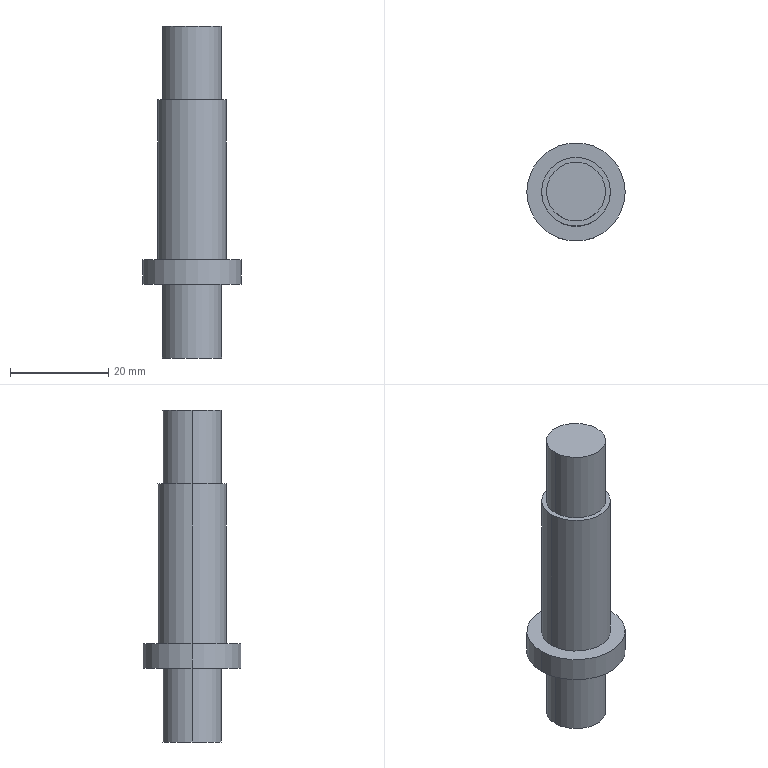Part | STEP file | Nylon handwheel shaft QY-1-37 | 1 solid | 13 faces | box 20 x 20 x 67.5 mm | volume 9967 mm3 | cylinder 8 | plane 5 | commonest cylinder face diameters 12 x4 14 x2 20 x2
STEP:
#1=CARTESIAN_POINT('',(0.,0.,0.));
#2=DIRECTION('',(0.,0.,1.));
#3=DIRECTION('',(1.,0.,0.));
#4=AXIS2_PLACEMENT_3D('',#1,#2,#3);
#5=CARTESIAN_POINT('',(-6.,0.,-20.));
#6=VERTEX_POINT('',#5);
#7=CARTESIAN_POINT('',(6.,0.,-20.));
#8=VERTEX_POINT('',#7);
#9=CARTESIAN_POINT('',(0.,0.,-20.));
#10=DIRECTION('',(0.,0.,-1.));
#11=DIRECTION('',(-1.,0.,0.));
#12=AXIS2_PLACEMENT_3D('',#9,#10,#11);
#13=CIRCLE('',#12,6.);
#14=CARTESIAN_POINT('',(0.,0.,-20.));
#15=DIRECTION('',(0.,0.,1.));
#16=DIRECTION('',(1.,0.,0.));
#17=AXIS2_PLACEMENT_3D('',#14,#15,#16);
#18=CYLINDRICAL_SURFACE('',#17,6.);
#19=CARTESIAN_POINT('',(3.142,0.));
#20=DIRECTION('',(-1.,0.));
#21=VECTOR('',#20,1.);
#22=LINE('',#19,#21);
#23=(GEOMETRIC_REPRESENTATION_CONTEXT(2)PARAMETRIC_REPRESENTATION_CONTEXT()REPRESENTATION_CONTEXT('',''));
#24=DEFINITIONAL_REPRESENTATION('',(#22),#23);
#25=PCURVE('',#18,#24);
#26=CARTESIAN_POINT('',(0.,0.,-20.));
#27=DIRECTION('',(0.,0.,-1.));
#28=DIRECTION('',(-1.,0.,0.));
#29=AXIS2_PLACEMENT_3D('',#26,#27,#28);
#30=PLANE('',#29);
#31=CARTESIAN_POINT('',(0.,0.));
#32=DIRECTION('',(1.,0.));
#33=AXIS2_PLACEMENT_2D('',#31,#32);
#34=CIRCLE('',#33,6.);
#35=(GEOMETRIC_REPRESENTATION_CONTEXT(2)PARAMETRIC_REPRESENTATION_CONTEXT()REPRESENTATION_CONTEXT('',''));
#36=DEFINITIONAL_REPRESENTATION('',(#34),#35);
#37=PCURVE('',#30,#36);
#38=SURFACE_CURVE('',#13,(#25,#37),.PCURVE_S1.);
#39=EDGE_CURVE('',#6,#8,#38,.T.);
#40=ORIENTED_EDGE('',*,*,#39,.F.);
#41=CARTESIAN_POINT('',(-6.,0.,-5.));
#42=VERTEX_POINT('',#41);
#43=CARTESIAN_POINT('',(-6.,0.,-20.));
#44=DIRECTION('',(0.,0.,1.));
#45=VECTOR('',#44,1.);
#46=LINE('',#43,#45);
#47=CARTESIAN_POINT('',(3.142,0.));
#48=DIRECTION('',(0.,1.));
#49=VECTOR('',#48,1.);
#50=LINE('',#47,#49);
#51=(GEOMETRIC_REPRESENTATION_CONTEXT(2)PARAMETRIC_REPRESENTATION_CONTEXT()REPRESENTATION_CONTEXT('',''));
#52=DEFINITIONAL_REPRESENTATION('',(#50),#51);
#53=PCURVE('',#18,#52);
#54=CARTESIAN_POINT('',(0.,0.,-20.));
#55=DIRECTION('',(0.,0.,1.));
#56=DIRECTION('',(1.,0.,0.));
#57=AXIS2_PLACEMENT_3D('',#54,#55,#56);
#58=CYLINDRICAL_SURFACE('',#57,6.);
#59=CARTESIAN_POINT('',(3.142,0.));
#60=DIRECTION('',(0.,1.));
#61=VECTOR('',#60,1.);
#62=LINE('',#59,#61);
#63=(GEOMETRIC_REPRESENTATION_CONTEXT(2)PARAMETRIC_REPRESENTATION_CONTEXT()REPRESENTATION_CONTEXT('',''));
#64=DEFINITIONAL_REPRESENTATION('',(#62),#63);
#65=PCURVE('',#58,#64);
#66=SURFACE_CURVE('',#46,(#53,#65),.PCURVE_S1.);
#67=EDGE_CURVE('',#6,#42,#66,.T.);
#68=ORIENTED_EDGE('',*,*,#67,.T.);
#69=CARTESIAN_POINT('',(6.,0.,-5.));
#70=VERTEX_POINT('',#69);
#71=CARTESIAN_POINT('',(0.,0.,-5.));
#72=DIRECTION('',(0.,0.,-1.));
#73=DIRECTION('',(-1.,0.,0.));
#74=AXIS2_PLACEMENT_3D('',#71,#72,#73);
#75=CIRCLE('',#74,6.);
#76=CARTESIAN_POINT('',(3.142,15.));
#77=DIRECTION('',(-1.,0.));
#78=VECTOR('',#77,1.);
#79=LINE('',#76,#78);
#80=(GEOMETRIC_REPRESENTATION_CONTEXT(2)PARAMETRIC_REPRESENTATION_CONTEXT()REPRESENTATION_CONTEXT('',''));
#81=DEFINITIONAL_REPRESENTATION('',(#79),#80);
#82=PCURVE('',#18,#81);
#83=CARTESIAN_POINT('',(0.,0.,-5.));
#84=DIRECTION('',(0.,0.,-1.));
#85=DIRECTION('',(-1.,0.,0.));
#86=AXIS2_PLACEMENT_3D('',#83,#84,#85);
#87=PLANE('',#86);
#88=CARTESIAN_POINT('',(0.,0.));
#89=DIRECTION('',(1.,0.));
#90=AXIS2_PLACEMENT_2D('',#88,#89);
#91=CIRCLE('',#90,6.);
#92=(GEOMETRIC_REPRESENTATION_CONTEXT(2)PARAMETRIC_REPRESENTATION_CONTEXT()REPRESENTATION_CONTEXT('',''));
#93=DEFINITIONAL_REPRESENTATION('',(#91),#92);
#94=PCURVE('',#87,#93);
#95=SURFACE_CURVE('',#75,(#82,#94),.PCURVE_S1.);
#96=EDGE_CURVE('',#42,#70,#95,.T.);
#97=ORIENTED_EDGE('',*,*,#96,.T.);
#98=CARTESIAN_POINT('',(6.,0.,-20.));
#99=DIRECTION('',(0.,0.,1.));
#100=VECTOR('',#99,1.);
#101=LINE('',#98,#100);
#102=CARTESIAN_POINT('',(0.,0.));
#103=DIRECTION('',(0.,1.));
#104=VECTOR('',#103,1.);
#105=LINE('',#102,#104);
#106=(GEOMETRIC_REPRESENTATION_CONTEXT(2)PARAMETRIC_REPRESENTATION_CONTEXT()REPRESENTATION_CONTEXT('',''));
#107=DEFINITIONAL_REPRESENTATION('',(#105),#106);
#108=PCURVE('',#18,#107);
#109=CARTESIAN_POINT('',(6.283,0.));
#110=DIRECTION('',(0.,1.));
#111=VECTOR('',#110,1.);
#112=LINE('',#109,#111);
#113=(GEOMETRIC_REPRESENTATION_CONTEXT(2)PARAMETRIC_REPRESENTATION_CONTEXT()REPRESENTATION_CONTEXT('',''));
#114=DEFINITIONAL_REPRESENTATION('',(#112),#113);
#115=PCURVE('',#58,#114);
#116=SURFACE_CURVE('',#101,(#108,#115),.PCURVE_S1.);
#117=EDGE_CURVE('',#8,#70,#116,.T.);
#118=ORIENTED_EDGE('',*,*,#117,.F.);
#119=EDGE_LOOP('',(#40,#68,#97,#118));
#120=FACE_BOUND('',#119,.T.);
#121=ADVANCED_FACE('',(#120),#18,.T.);
#122=CARTESIAN_POINT('',(-10.,0.,-5.));
#123=VERTEX_POINT('',#122);
#124=CARTESIAN_POINT('',(10.,0.,-5.));
#125=VERTEX_POINT('',#124);
#126=CARTESIAN_POINT('',(0.,0.,-5.));
#127=DIRECTION('',(0.,0.,-1.));
#128=DIRECTION('',(-1.,0.,0.));
#129=AXIS2_PLACEMENT_3D('',#126,#127,#128);
#130=CIRCLE('',#129,10.);
#131=CARTESIAN_POINT('',(0.,0.,-5.));
#132=DIRECTION('',(0.,0.,1.));
#133=DIRECTION('',(1.,0.,0.));
#134=AXIS2_PLACEMENT_3D('',#131,#132,#133);
#135=CYLINDRICAL_SURFACE('',#134,10.);
#136=CARTESIAN_POINT('',(3.142,0.));
#137=DIRECTION('',(-1.,0.));
#138=VECTOR('',#137,1.);
#139=LINE('',#136,#138);
#140=(GEOMETRIC_REPRESENTATION_CONTEXT(2)PARAMETRIC_REPRESENTATION_CONTEXT()REPRESENTATION_CONTEXT('',''));
#141=DEFINITIONAL_REPRESENTATION('',(#139),#140);
#142=PCURVE('',#135,#141);
#143=CARTESIAN_POINT('',(0.,0.));
#144=DIRECTION('',(1.,0.));
#145=AXIS2_PLACEMENT_2D('',#143,#144);
#146=CIRCLE('',#145,10.);
#147=(GEOMETRIC_REPRESENTATION_CONTEXT(2)PARAMETRIC_REPRESENTATION_CONTEXT()REPRESENTATION_CONTEXT('',''));
#148=DEFINITIONAL_REPRESENTATION('',(#146),#147);
#149=PCURVE('',#87,#148);
#150=SURFACE_CURVE('',#130,(#142,#149),.PCURVE_S1.);
#151=EDGE_CURVE('',#123,#125,#150,.T.);
#152=ORIENTED_EDGE('',*,*,#151,.F.);
#153=CARTESIAN_POINT('',(-10.,0.,0.));
#154=VERTEX_POINT('',#153);
#155=CARTESIAN_POINT('',(-10.,0.,-5.));
#156=DIRECTION('',(0.,0.,1.));
#157=VECTOR('',#156,1.);
#158=LINE('',#155,#157);
#159=CARTESIAN_POINT('',(3.142,0.));
#160=DIRECTION('',(0.,1.));
#161=VECTOR('',#160,1.);
#162=LINE('',#159,#161);
#163=(GEOMETRIC_REPRESENTATION_CONTEXT(2)PARAMETRIC_REPRESENTATION_CONTEXT()REPRESENTATION_CONTEXT('',''));
#164=DEFINITIONAL_REPRESENTATION('',(#162),#163);
#165=PCURVE('',#135,#164);
#166=CARTESIAN_POINT('',(0.,0.,-5.));
#167=DIRECTION('',(0.,0.,1.));
#168=DIRECTION('',(1.,0.,0.));
#169=AXIS2_PLACEMENT_3D('',#166,#167,#168);
#170=CYLINDRICAL_SURFACE('',#169,10.);
#171=CARTESIAN_POINT('',(3.142,0.));
#172=DIRECTION('',(0.,1.));
#173=VECTOR('',#172,1.);
#174=LINE('',#171,#173);
#175=(GEOMETRIC_REPRESENTATION_CONTEXT(2)PARAMETRIC_REPRESENTATION_CONTEXT()REPRESENTATION_CONTEXT('',''));
#176=DEFINITIONAL_REPRESENTATION('',(#174),#175);
#177=PCURVE('',#170,#176);
#178=SURFACE_CURVE('',#158,(#165,#177),.PCURVE_S1.);
#179=EDGE_CURVE('',#123,#154,#178,.T.);
#180=ORIENTED_EDGE('',*,*,#179,.T.);
#181=CARTESIAN_POINT('',(10.,0.,0.));
#182=VERTEX_POINT('',#181);
#183=CARTESIAN_POINT('',(0.,0.,0.));
#184=DIRECTION('',(0.,0.,-1.));
#185=DIRECTION('',(-1.,0.,0.));
#186=AXIS2_PLACEMENT_3D('',#183,#184,#185);
#187=CIRCLE('',#186,10.);
#188=CARTESIAN_POINT('',(3.142,5.));
#189=DIRECTION('',(-1.,0.));
#190=VECTOR('',#189,1.);
#191=LINE('',#188,#190);
#192=(GEOMETRIC_REPRESENTATION_CONTEXT(2)PARAMETRIC_REPRESENTATION_CONTEXT()REPRESENTATION_CONTEXT('',''));
#193=DEFINITIONAL_REPRESENTATION('',(#191),#192);
#194=PCURVE('',#135,#193);
#195=CARTESIAN_POINT('',(0.,0.,0.));
#196=DIRECTION('',(0.,0.,-1.));
#197=DIRECTION('',(-1.,0.,0.));
#198=AXIS2_PLACEMENT_3D('',#195,#196,#197);
#199=PLANE('',#198);
#200=CARTESIAN_POINT('',(0.,0.));
#201=DIRECTION('',(1.,0.));
#202=AXIS2_PLACEMENT_2D('',#200,#201);
#203=CIRCLE('',#202,10.);
#204=(GEOMETRIC_REPRESENTATION_CONTEXT(2)PARAMETRIC_REPRESENTATION_CONTEXT()REPRESENTATION_CONTEXT('',''));
#205=DEFINITIONAL_REPRESENTATION('',(#203),#204);
#206=PCURVE('',#199,#205);
#207=SURFACE_CURVE('',#187,(#194,#206),.PCURVE_S1.);
#208=EDGE_CURVE('',#154,#182,#207,.T.);
#209=ORIENTED_EDGE('',*,*,#208,.T.);
#210=CARTESIAN_POINT('',(10.,0.,-5.));
#211=DIRECTION('',(0.,0.,1.));
#212=VECTOR('',#211,1.);
#213=LINE('',#210,#212);
#214=CARTESIAN_POINT('',(0.,0.));
#215=DIRECTION('',(0.,1.));
#216=VECTOR('',#215,1.);
#217=LINE('',#214,#216);
#218=(GEOMETRIC_REPRESENTATION_CONTEXT(2)PARAMETRIC_REPRESENTATION_CONTEXT()REPRESENTATION_CONTEXT('',''));
#219=DEFINITIONAL_REPRESENTATION('',(#217),#218);
#220=PCURVE('',#135,#219);
#221=CARTESIAN_POINT('',(6.283,0.));
#222=DIRECTION('',(0.,1.));
#223=VECTOR('',#222,1.);
#224=LINE('',#221,#223);
#225=(GEOMETRIC_REPRESENTATION_CONTEXT(2)PARAMETRIC_REPRESENTATION_CONTEXT()REPRESENTATION_CONTEXT('',''));
#226=DEFINITIONAL_REPRESENTATION('',(#224),#225);
#227=PCURVE('',#170,#226);
#228=SURFACE_CURVE('',#213,(#220,#227),.PCURVE_S1.);
#229=EDGE_CURVE('',#125,#182,#228,.T.);
#230=ORIENTED_EDGE('',*,*,#229,.F.);
#231=EDGE_LOOP('',(#152,#180,#209,#230));
#232=FACE_BOUND('',#231,.T.);
#233=ADVANCED_FACE('',(#232),#135,.T.);
#234=CARTESIAN_POINT('',(6.,0.,47.5));
#235=VERTEX_POINT('',#234);
#236=CARTESIAN_POINT('',(-6.,0.,47.5));
#237=VERTEX_POINT('',#236);
#238=CARTESIAN_POINT('',(0.,0.,47.5));
#239=DIRECTION('',(0.,0.,1.));
#240=DIRECTION('',(1.,0.,0.));
#241=AXIS2_PLACEMENT_3D('',#238,#239,#240);
#242=CIRCLE('',#241,6.);
#243=CARTESIAN_POINT('',(0.,0.,47.5));
#244=DIRECTION('',(0.,0.,-1.));
#245=DIRECTION('',(-1.,0.,0.));
#246=AXIS2_PLACEMENT_3D('',#243,#244,#245);
#247=CYLINDRICAL_SURFACE('',#246,6.);
#248=CARTESIAN_POINT('',(3.142,0.));
#249=DIRECTION('',(-1.,0.));
#250=VECTOR('',#249,1.);
#251=LINE('',#248,#250);
#252=(GEOMETRIC_REPRESENTATION_CONTEXT(2)PARAMETRIC_REPRESENTATION_CONTEXT()REPRESENTATION_CONTEXT('',''));
#253=DEFINITIONAL_REPRESENTATION('',(#251),#252);
#254=PCURVE('',#247,#253);
#255=CARTESIAN_POINT('',(0.,0.,47.5));
#256=DIRECTION('',(0.,0.,1.));
#257=DIRECTION('',(1.,0.,0.));
#258=AXIS2_PLACEMENT_3D('',#255,#256,#257);
#259=PLANE('',#258);
#260=CARTESIAN_POINT('',(0.,0.));
#261=DIRECTION('',(1.,0.));
#262=AXIS2_PLACEMENT_2D('',#260,#261);
#263=CIRCLE('',#262,6.);
#264=(GEOMETRIC_REPRESENTATION_CONTEXT(2)PARAMETRIC_REPRESENTATION_CONTEXT()REPRESENTATION_CONTEXT('',''));
#265=DEFINITIONAL_REPRESENTATION('',(#263),#264);
#266=PCURVE('',#259,#265);
#267=SURFACE_CURVE('',#242,(#254,#266),.PCURVE_S1.);
#268=EDGE_CURVE('',#235,#237,#267,.T.);
#269=ORIENTED_EDGE('',*,*,#268,.F.);
#270=CARTESIAN_POINT('',(6.,0.,32.5));
#271=VERTEX_POINT('',#270);
#272=CARTESIAN_POINT('',(6.,0.,47.5));
#273=DIRECTION('',(0.,0.,-1.));
#274=VECTOR('',#273,1.);
#275=LINE('',#272,#274);
#276=CARTESIAN_POINT('',(3.142,0.));
#277=DIRECTION('',(0.,1.));
#278=VECTOR('',#277,1.);
#279=LINE('',#276,#278);
#280=(GEOMETRIC_REPRESENTATION_CONTEXT(2)PARAMETRIC_REPRESENTATION_CONTEXT()REPRESENTATION_CONTEXT('',''));
#281=DEFINITIONAL_REPRESENTATION('',(#279),#280);
#282=PCURVE('',#247,#281);
#283=CARTESIAN_POINT('',(0.,0.,47.5));
#284=DIRECTION('',(0.,0.,-1.));
#285=DIRECTION('',(-1.,0.,0.));
#286=AXIS2_PLACEMENT_3D('',#283,#284,#285);
#287=CYLINDRICAL_SURFACE('',#286,6.);
#288=CARTESIAN_POINT('',(3.142,0.));
#289=DIRECTION('',(0.,1.));
#290=VECTOR('',#289,1.);
#291=LINE('',#288,#290);
#292=(GEOMETRIC_REPRESENTATION_CONTEXT(2)PARAMETRIC_REPRESENTATION_CONTEXT()REPRESENTATION_CONTEXT('',''));
#293=DEFINITIONAL_REPRESENTATION('',(#291),#292);
#294=PCURVE('',#287,#293);
#295=SURFACE_CURVE('',#275,(#282,#294),.PCURVE_S1.);
#296=EDGE_CURVE('',#235,#271,#295,.T.);
#297=ORIENTED_EDGE('',*,*,#296,.T.);
#298=CARTESIAN_POINT('',(-6.,0.,32.5));
#299=VERTEX_POINT('',#298);
#300=CARTESIAN_POINT('',(0.,0.,32.5));
#301=DIRECTION('',(0.,0.,1.));
#302=DIRECTION('',(1.,0.,0.));
#303=AXIS2_PLACEMENT_3D('',#300,#301,#302);
#304=CIRCLE('',#303,6.);
#305=CARTESIAN_POINT('',(3.142,15.));
#306=DIRECTION('',(-1.,0.));
#307=VECTOR('',#306,1.);
#308=LINE('',#305,#307);
#309=(GEOMETRIC_REPRESENTATION_CONTEXT(2)PARAMETRIC_REPRESENTATION_CONTEXT()REPRESENTATION_CONTEXT('',''));
#310=DEFINITIONAL_REPRESENTATION('',(#308),#309);
#311=PCURVE('',#247,#310);
#312=CARTESIAN_POINT('',(0.,0.,32.5));
#313=DIRECTION('',(0.,0.,1.));
#314=DIRECTION('',(1.,0.,0.));
#315=AXIS2_PLACEMENT_3D('',#312,#313,#314);
#316=PLANE('',#315);
#317=CARTESIAN_POINT('',(0.,0.));
#318=DIRECTION('',(1.,0.));
#319=AXIS2_PLACEMENT_2D('',#317,#318);
#320=CIRCLE('',#319,6.);
#321=(GEOMETRIC_REPRESENTATION_CONTEXT(2)PARAMETRIC_REPRESENTATION_CONTEXT()REPRESENTATION_CONTEXT('',''));
#322=DEFINITIONAL_REPRESENTATION('',(#320),#321);
#323=PCURVE('',#316,#322);
#324=SURFACE_CURVE('',#304,(#311,#323),.PCURVE_S1.);
#325=EDGE_CURVE('',#271,#299,#324,.T.);
#326=ORIENTED_EDGE('',*,*,#325,.T.);
#327=CARTESIAN_POINT('',(-6.,0.,47.5));
#328=DIRECTION('',(0.,0.,-1.));
#329=VECTOR('',#328,1.);
#330=LINE('',#327,#329);
#331=CARTESIAN_POINT('',(0.,0.));
#332=DIRECTION('',(0.,1.));
#333=VECTOR('',#332,1.);
#334=LINE('',#331,#333);
#335=(GEOMETRIC_REPRESENTATION_CONTEXT(2)PARAMETRIC_REPRESENTATION_CONTEXT()REPRESENTATION_CONTEXT('',''));
#336=DEFINITIONAL_REPRESENTATION('',(#334),#335);
#337=PCURVE('',#247,#336);
#338=CARTESIAN_POINT('',(6.283,0.));
#339=DIRECTION('',(0.,1.));
#340=VECTOR('',#339,1.);
#341=LINE('',#338,#340);
#342=(GEOMETRIC_REPRESENTATION_CONTEXT(2)PARAMETRIC_REPRESENTATION_CONTEXT()REPRESENTATION_CONTEXT('',''));
#343=DEFINITIONAL_REPRESENTATION('',(#341),#342);
#344=PCURVE('',#287,#343);
#345=SURFACE_CURVE('',#330,(#337,#344),.PCURVE_S1.);
#346=EDGE_CURVE('',#237,#299,#345,.T.);
#347=ORIENTED_EDGE('',*,*,#346,.F.);
#348=EDGE_LOOP('',(#269,#297,#326,#347));
#349=FACE_BOUND('',#348,.T.);
#350=ADVANCED_FACE('',(#349),#247,.T.);
#351=CARTESIAN_POINT('',(7.,0.,32.5));
#352=VERTEX_POINT('',#351);
#353=CARTESIAN_POINT('',(-7.,0.,32.5));
#354=VERTEX_POINT('',#353);
#355=CARTESIAN_POINT('',(0.,0.,32.5));
#356=DIRECTION('',(0.,0.,1.));
#357=DIRECTION('',(1.,0.,0.));
#358=AXIS2_PLACEMENT_3D('',#355,#356,#357);
#359=CIRCLE('',#358,7.);
#360=CARTESIAN_POINT('',(0.,0.,32.5));
#361=DIRECTION('',(0.,0.,-1.));
#362=DIRECTION('',(-1.,0.,0.));
#363=AXIS2_PLACEMENT_3D('',#360,#361,#362);
#364=CYLINDRICAL_SURFACE('',#363,7.);
#365=CARTESIAN_POINT('',(3.142,0.));
#366=DIRECTION('',(-1.,0.));
#367=VECTOR('',#366,1.);
#368=LINE('',#365,#367);
#369=(GEOMETRIC_REPRESENTATION_CONTEXT(2)PARAMETRIC_REPRESENTATION_CONTEXT()REPRESENTATION_CONTEXT('',''));
#370=DEFINITIONAL_REPRESENTATION('',(#368),#369);
#371=PCURVE('',#364,#370);
#372=CARTESIAN_POINT('',(0.,0.));
#373=DIRECTION('',(1.,0.));
#374=AXIS2_PLACEMENT_2D('',#372,#373);
#375=CIRCLE('',#374,7.);
#376=(GEOMETRIC_REPRESENTATION_CONTEXT(2)PARAMETRIC_REPRESENTATION_CONTEXT()REPRESENTATION_CONTEXT('',''));
#377=DEFINITIONAL_REPRESENTATION('',(#375),#376);
#378=PCURVE('',#316,#377);
#379=SURFACE_CURVE('',#359,(#371,#378),.PCURVE_S1.);
#380=EDGE_CURVE('',#352,#354,#379,.T.);
#381=ORIENTED_EDGE('',*,*,#380,.F.);
#382=CARTESIAN_POINT('',(7.,0.,0.));
#383=VERTEX_POINT('',#382);
#384=CARTESIAN_POINT('',(7.,0.,32.5));
#385=DIRECTION('',(0.,0.,-1.));
#386=VECTOR('',#385,1.);
#387=LINE('',#384,#386);
#388=CARTESIAN_POINT('',(3.142,0.));
#389=DIRECTION('',(0.,1.));
#390=VECTOR('',#389,1.);
#391=LINE('',#388,#390);
#392=(GEOMETRIC_REPRESENTATION_CONTEXT(2)PARAMETRIC_REPRESENTATION_CONTEXT()REPRESENTATION_CONTEXT('',''));
#393=DEFINITIONAL_REPRESENTATION('',(#391),#392);
#394=PCURVE('',#364,#393);
#395=CARTESIAN_POINT('',(0.,0.,32.5));
#396=DIRECTION('',(0.,0.,-1.));
#397=DIRECTION('',(-1.,0.,0.));
#398=AXIS2_PLACEMENT_3D('',#395,#396,#397);
#399=CYLINDRICAL_SURFACE('',#398,7.);
#400=CARTESIAN_POINT('',(3.142,0.));
#401=DIRECTION('',(0.,1.));
#402=VECTOR('',#401,1.);
#403=LINE('',#400,#402);
#404=(GEOMETRIC_REPRESENTATION_CONTEXT(2)PARAMETRIC_REPRESENTATION_CONTEXT()REPRESENTATION_CONTEXT('',''));
#405=DEFINITIONAL_REPRESENTATION('',(#403),#404);
#406=PCURVE('',#399,#405);
#407=SURFACE_CURVE('',#387,(#394,#406),.PCURVE_S1.);
#408=EDGE_CURVE('',#352,#383,#407,.T.);
#409=ORIENTED_EDGE('',*,*,#408,.T.);
#410=CARTESIAN_POINT('',(-7.,0.,0.));
#411=VERTEX_POINT('',#410);
#412=CARTESIAN_POINT('',(0.,0.,0.));
#413=DIRECTION('',(0.,0.,1.));
#414=DIRECTION('',(1.,0.,0.));
#415=AXIS2_PLACEMENT_3D('',#412,#413,#414);
#416=CIRCLE('',#415,7.);
#417=CARTESIAN_POINT('',(3.142,32.5));
#418=DIRECTION('',(-1.,0.));
#419=VECTOR('',#418,1.);
#420=LINE('',#417,#419);
#421=(GEOMETRIC_REPRESENTATION_CONTEXT(2)PARAMETRIC_REPRESENTATION_CONTEXT()REPRESENTATION_CONTEXT('',''));
#422=DEFINITIONAL_REPRESENTATION('',(#420),#421);
#423=PCURVE('',#364,#422);
#424=CARTESIAN_POINT('',(-7.,0.));
#425=CARTESIAN_POINT('',(-7.,12.124));
#426=CARTESIAN_POINT('',(3.5,6.062));
#427=CARTESIAN_POINT('',(14.,0.));
#428=CARTESIAN_POINT('',(3.5,-6.062));
#429=CARTESIAN_POINT('',(-7.,-12.124));
#430=CARTESIAN_POINT('',(-7.,0.));
#431=(BOUNDED_CURVE()B_SPLINE_CURVE(2,(#424,#425,#426,#427,#428,#429,#430),.UNSPECIFIED.,.T.,.F.)B_SPLINE_CURVE_WITH_KNOTS((1,2,2,2,2,1),(-2.094,0.,2.094,4.189,6.283,8.378),.UNSPECIFIED.)CURVE()GEOMETRIC_REPRESENTATION_ITEM()RATIONAL_B_SPLINE_CURVE((1.,0.5,1.,0.5,1.,0.5,1.))REPRESENTATION_ITEM(''));
#432=(GEOMETRIC_REPRESENTATION_CONTEXT(2)PARAMETRIC_REPRESENTATION_CONTEXT()REPRESENTATION_CONTEXT('',''));
#433=DEFINITIONAL_REPRESENTATION('',(#431),#432);
#434=PCURVE('',#199,#433);
#435=SURFACE_CURVE('',#416,(#423,#434),.PCURVE_S1.);
#436=EDGE_CURVE('',#383,#411,#435,.T.);
#437=ORIENTED_EDGE('',*,*,#436,.T.);
#438=CARTESIAN_POINT('',(-7.,0.,32.5));
#439=DIRECTION('',(0.,0.,-1.));
#440=VECTOR('',#439,1.);
#441=LINE('',#438,#440);
#442=CARTESIAN_POINT('',(0.,0.));
#443=DIRECTION('',(0.,1.));
#444=VECTOR('',#443,1.);
#445=LINE('',#442,#444);
#446=(GEOMETRIC_REPRESENTATION_CONTEXT(2)PARAMETRIC_REPRESENTATION_CONTEXT()REPRESENTATION_CONTEXT('',''));
#447=DEFINITIONAL_REPRESENTATION('',(#445),#446);
#448=PCURVE('',#364,#447);
#449=CARTESIAN_POINT('',(6.283,0.));
#450=DIRECTION('',(0.,1.));
#451=VECTOR('',#450,1.);
#452=LINE('',#449,#451);
#453=(GEOMETRIC_REPRESENTATION_CONTEXT(2)PARAMETRIC_REPRESENTATION_CONTEXT()REPRESENTATION_CONTEXT('',''));
#454=DEFINITIONAL_REPRESENTATION('',(#452),#453);
#455=PCURVE('',#399,#454);
#456=SURFACE_CURVE('',#441,(#448,#455),.PCURVE_S1.);
#457=EDGE_CURVE('',#354,#411,#456,.T.);
#458=ORIENTED_EDGE('',*,*,#457,.F.);
#459=EDGE_LOOP('',(#381,#409,#437,#458));
#460=FACE_BOUND('',#459,.T.);
#461=ADVANCED_FACE('',(#460),#364,.T.);
#462=ORIENTED_EDGE('',*,*,#408,.F.);
#463=CARTESIAN_POINT('',(0.,0.,32.5));
#464=DIRECTION('',(0.,0.,1.));
#465=DIRECTION('',(1.,0.,0.));
#466=AXIS2_PLACEMENT_3D('',#463,#464,#465);
#467=CIRCLE('',#466,7.);
#468=CARTESIAN_POINT('',(9.425,0.));
#469=DIRECTION('',(-1.,0.));
#470=VECTOR('',#469,1.);
#471=LINE('',#468,#470);
#472=(GEOMETRIC_REPRESENTATION_CONTEXT(2)PARAMETRIC_REPRESENTATION_CONTEXT()REPRESENTATION_CONTEXT('',''));
#473=DEFINITIONAL_REPRESENTATION('',(#471),#472);
#474=PCURVE('',#399,#473);
#475=CARTESIAN_POINT('',(0.,0.));
#476=DIRECTION('',(1.,0.));
#477=AXIS2_PLACEMENT_2D('',#475,#476);
#478=CIRCLE('',#477,7.);
#479=(GEOMETRIC_REPRESENTATION_CONTEXT(2)PARAMETRIC_REPRESENTATION_CONTEXT()REPRESENTATION_CONTEXT('',''));
#480=DEFINITIONAL_REPRESENTATION('',(#478),#479);
#481=PCURVE('',#316,#480);
#482=SURFACE_CURVE('',#467,(#474,#481),.PCURVE_S1.);
#483=EDGE_CURVE('',#354,#352,#482,.T.);
#484=ORIENTED_EDGE('',*,*,#483,.F.);
#485=ORIENTED_EDGE('',*,*,#457,.T.);
#486=CARTESIAN_POINT('',(0.,0.,0.));
#487=DIRECTION('',(0.,0.,1.));
#488=DIRECTION('',(1.,0.,0.));
#489=AXIS2_PLACEMENT_3D('',#486,#487,#488);
#490=CIRCLE('',#489,7.);
#491=CARTESIAN_POINT('',(9.425,32.5));
#492=DIRECTION('',(-1.,0.));
#493=VECTOR('',#492,1.);
#494=LINE('',#491,#493);
#495=(GEOMETRIC_REPRESENTATION_CONTEXT(2)PARAMETRIC_REPRESENTATION_CONTEXT()REPRESENTATION_CONTEXT('',''));
#496=DEFINITIONAL_REPRESENTATION('',(#494),#495);
#497=PCURVE('',#399,#496);
#498=CARTESIAN_POINT('',(-7.,0.));
#499=CARTESIAN_POINT('',(-7.,12.124));
#500=CARTESIAN_POINT('',(3.5,6.062));
#501=CARTESIAN_POINT('',(14.,0.));
#502=CARTESIAN_POINT('',(3.5,-6.062));
#503=CARTESIAN_POINT('',(-7.,-12.124));
#504=CARTESIAN_POINT('',(-7.,0.));
#505=(BOUNDED_CURVE()B_SPLINE_CURVE(2,(#498,#499,#500,#501,#502,#503,#504),.UNSPECIFIED.,.T.,.F.)B_SPLINE_CURVE_WITH_KNOTS((1,2,2,2,2,1),(-2.094,0.,2.094,4.189,6.283,8.378),.UNSPECIFIED.)CURVE()GEOMETRIC_REPRESENTATION_ITEM()RATIONAL_B_SPLINE_CURVE((1.,0.5,1.,0.5,1.,0.5,1.))REPRESENTATION_ITEM(''));
#506=(GEOMETRIC_REPRESENTATION_CONTEXT(2)PARAMETRIC_REPRESENTATION_CONTEXT()REPRESENTATION_CONTEXT('',''));
#507=DEFINITIONAL_REPRESENTATION('',(#505),#506);
#508=PCURVE('',#199,#507);
#509=SURFACE_CURVE('',#490,(#497,#508),.PCURVE_S1.);
#510=EDGE_CURVE('',#411,#383,#509,.T.);
#511=ORIENTED_EDGE('',*,*,#510,.T.);
#512=EDGE_LOOP('',(#462,#484,#485,#511));
#513=FACE_BOUND('',#512,.T.);
#514=ADVANCED_FACE('',(#513),#399,.T.);
#515=CARTESIAN_POINT('',(0.,0.,32.5));
#516=DIRECTION('',(0.,0.,1.));
#517=DIRECTION('',(1.,0.,0.));
#518=AXIS2_PLACEMENT_3D('',#515,#516,#517);
#519=CIRCLE('',#518,6.);
#520=CARTESIAN_POINT('',(0.,0.));
#521=DIRECTION('',(1.,0.));
#522=AXIS2_PLACEMENT_2D('',#520,#521);
#523=CIRCLE('',#522,6.);
#524=(GEOMETRIC_REPRESENTATION_CONTEXT(2)PARAMETRIC_REPRESENTATION_CONTEXT()REPRESENTATION_CONTEXT('',''));
#525=DEFINITIONAL_REPRESENTATION('',(#523),#524);
#526=PCURVE('',#316,#525);
#527=CARTESIAN_POINT('',(9.425,15.));
#528=DIRECTION('',(-1.,0.));
#529=VECTOR('',#528,1.);
#530=LINE('',#527,#529);
#531=(GEOMETRIC_REPRESENTATION_CONTEXT(2)PARAMETRIC_REPRESENTATION_CONTEXT()REPRESENTATION_CONTEXT('',''));
#532=DEFINITIONAL_REPRESENTATION('',(#530),#531);
#533=PCURVE('',#287,#532);
#534=SURFACE_CURVE('',#519,(#526,#533),.PCURVE_S1.);
#535=EDGE_CURVE('',#299,#271,#534,.T.);
#536=ORIENTED_EDGE('',*,*,#535,.F.);
#537=ORIENTED_EDGE('',*,*,#325,.F.);
#538=EDGE_LOOP('',(#536,#537));
#539=FACE_BOUND('',#538,.T.);
#540=ORIENTED_EDGE('',*,*,#483,.T.);
#541=ORIENTED_EDGE('',*,*,#380,.T.);
#542=EDGE_LOOP('',(#540,#541));
#543=FACE_BOUND('',#542,.T.);
#544=ADVANCED_FACE('',(#539,#543),#316,.T.);
#545=ORIENTED_EDGE('',*,*,#296,.F.);
#546=CARTESIAN_POINT('',(0.,0.,47.5));
#547=DIRECTION('',(0.,0.,1.));
#548=DIRECTION('',(1.,0.,0.));
#549=AXIS2_PLACEMENT_3D('',#546,#547,#548);
#550=CIRCLE('',#549,6.);
#551=CARTESIAN_POINT('',(9.425,0.));
#552=DIRECTION('',(-1.,0.));
#553=VECTOR('',#552,1.);
#554=LINE('',#551,#553);
#555=(GEOMETRIC_REPRESENTATION_CONTEXT(2)PARAMETRIC_REPRESENTATION_CONTEXT()REPRESENTATION_CONTEXT('',''));
#556=DEFINITIONAL_REPRESENTATION('',(#554),#555);
#557=PCURVE('',#287,#556);
#558=CARTESIAN_POINT('',(0.,0.));
#559=DIRECTION('',(1.,0.));
#560=AXIS2_PLACEMENT_2D('',#558,#559);
#561=CIRCLE('',#560,6.);
#562=(GEOMETRIC_REPRESENTATION_CONTEXT(2)PARAMETRIC_REPRESENTATION_CONTEXT()REPRESENTATION_CONTEXT('',''));
#563=DEFINITIONAL_REPRESENTATION('',(#561),#562);
#564=PCURVE('',#259,#563);
#565=SURFACE_CURVE('',#550,(#557,#564),.PCURVE_S1.);
#566=EDGE_CURVE('',#237,#235,#565,.T.);
#567=ORIENTED_EDGE('',*,*,#566,.F.);
#568=ORIENTED_EDGE('',*,*,#346,.T.);
#569=ORIENTED_EDGE('',*,*,#535,.T.);
#570=EDGE_LOOP('',(#545,#567,#568,#569));
#571=FACE_BOUND('',#570,.T.);
#572=ADVANCED_FACE('',(#571),#287,.T.);
#573=ORIENTED_EDGE('',*,*,#566,.T.);
#574=ORIENTED_EDGE('',*,*,#268,.T.);
#575=EDGE_LOOP('',(#573,#574));
#576=FACE_BOUND('',#575,.T.);
#577=ADVANCED_FACE('',(#576),#259,.T.);
#578=ORIENTED_EDGE('',*,*,#179,.F.);
#579=CARTESIAN_POINT('',(0.,0.,-5.));
#580=DIRECTION('',(0.,0.,-1.));
#581=DIRECTION('',(-1.,0.,0.));
#582=AXIS2_PLACEMENT_3D('',#579,#580,#581);
#583=CIRCLE('',#582,10.);
#584=CARTESIAN_POINT('',(9.425,0.));
#585=DIRECTION('',(-1.,0.));
#586=VECTOR('',#585,1.);
#587=LINE('',#584,#586);
#588=(GEOMETRIC_REPRESENTATION_CONTEXT(2)PARAMETRIC_REPRESENTATION_CONTEXT()REPRESENTATION_CONTEXT('',''));
#589=DEFINITIONAL_REPRESENTATION('',(#587),#588);
#590=PCURVE('',#170,#589);
#591=CARTESIAN_POINT('',(0.,0.));
#592=DIRECTION('',(1.,0.));
#593=AXIS2_PLACEMENT_2D('',#591,#592);
#594=CIRCLE('',#593,10.);
#595=(GEOMETRIC_REPRESENTATION_CONTEXT(2)PARAMETRIC_REPRESENTATION_CONTEXT()REPRESENTATION_CONTEXT('',''));
#596=DEFINITIONAL_REPRESENTATION('',(#594),#595);
#597=PCURVE('',#87,#596);
#598=SURFACE_CURVE('',#583,(#590,#597),.PCURVE_S1.);
#599=EDGE_CURVE('',#125,#123,#598,.T.);
#600=ORIENTED_EDGE('',*,*,#599,.F.);
#601=ORIENTED_EDGE('',*,*,#229,.T.);
#602=CARTESIAN_POINT('',(0.,0.,0.));
#603=DIRECTION('',(0.,0.,-1.));
#604=DIRECTION('',(-1.,0.,0.));
#605=AXIS2_PLACEMENT_3D('',#602,#603,#604);
#606=CIRCLE('',#605,10.);
#607=CARTESIAN_POINT('',(9.425,5.));
#608=DIRECTION('',(-1.,0.));
#609=VECTOR('',#608,1.);
#610=LINE('',#607,#609);
#611=(GEOMETRIC_REPRESENTATION_CONTEXT(2)PARAMETRIC_REPRESENTATION_CONTEXT()REPRESENTATION_CONTEXT('',''));
#612=DEFINITIONAL_REPRESENTATION('',(#610),#611);
#613=PCURVE('',#170,#612);
#614=CARTESIAN_POINT('',(0.,0.));
#615=DIRECTION('',(1.,0.));
#616=AXIS2_PLACEMENT_2D('',#614,#615);
#617=CIRCLE('',#616,10.);
#618=(GEOMETRIC_REPRESENTATION_CONTEXT(2)PARAMETRIC_REPRESENTATION_CONTEXT()REPRESENTATION_CONTEXT('',''));
#619=DEFINITIONAL_REPRESENTATION('',(#617),#618);
#620=PCURVE('',#199,#619);
#621=SURFACE_CURVE('',#606,(#613,#620),.PCURVE_S1.);
#622=EDGE_CURVE('',#182,#154,#621,.T.);
#623=ORIENTED_EDGE('',*,*,#622,.T.);
#624=EDGE_LOOP('',(#578,#600,#601,#623));
#625=FACE_BOUND('',#624,.T.);
#626=ADVANCED_FACE('',(#625),#170,.T.);
#627=CARTESIAN_POINT('',(0.,0.,-5.));
#628=DIRECTION('',(0.,0.,-1.));
#629=DIRECTION('',(-1.,0.,0.));
#630=AXIS2_PLACEMENT_3D('',#627,#628,#629);
#631=CIRCLE('',#630,6.);
#632=CARTESIAN_POINT('',(0.,0.));
#633=DIRECTION('',(1.,0.));
#634=AXIS2_PLACEMENT_2D('',#632,#633);
#635=CIRCLE('',#634,6.);
#636=(GEOMETRIC_REPRESENTATION_CONTEXT(2)PARAMETRIC_REPRESENTATION_CONTEXT()REPRESENTATION_CONTEXT('',''));
#637=DEFINITIONAL_REPRESENTATION('',(#635),#636);
#638=PCURVE('',#87,#637);
#639=CARTESIAN_POINT('',(9.425,15.));
#640=DIRECTION('',(-1.,0.));
#641=VECTOR('',#640,1.);
#642=LINE('',#639,#641);
#643=(GEOMETRIC_REPRESENTATION_CONTEXT(2)PARAMETRIC_REPRESENTATION_CONTEXT()REPRESENTATION_CONTEXT('',''));
#644=DEFINITIONAL_REPRESENTATION('',(#642),#643);
#645=PCURVE('',#58,#644);
#646=SURFACE_CURVE('',#631,(#638,#645),.PCURVE_S1.);
#647=EDGE_CURVE('',#70,#42,#646,.T.);
#648=ORIENTED_EDGE('',*,*,#647,.F.);
#649=ORIENTED_EDGE('',*,*,#96,.F.);
#650=EDGE_LOOP('',(#648,#649));
#651=FACE_BOUND('',#650,.T.);
#652=ORIENTED_EDGE('',*,*,#599,.T.);
#653=ORIENTED_EDGE('',*,*,#151,.T.);
#654=EDGE_LOOP('',(#652,#653));
#655=FACE_BOUND('',#654,.T.);
#656=ADVANCED_FACE('',(#651,#655),#87,.T.);
#657=ORIENTED_EDGE('',*,*,#510,.F.);
#658=ORIENTED_EDGE('',*,*,#436,.F.);
#659=EDGE_LOOP('',(#657,#658));
#660=FACE_BOUND('',#659,.T.);
#661=ORIENTED_EDGE('',*,*,#622,.F.);
#662=ORIENTED_EDGE('',*,*,#208,.F.);
#663=EDGE_LOOP('',(#661,#662));
#664=FACE_BOUND('',#663,.T.);
#665=ADVANCED_FACE('',(#660,#664),#199,.F.);
#666=ORIENTED_EDGE('',*,*,#67,.F.);
#667=CARTESIAN_POINT('',(0.,0.,-20.));
#668=DIRECTION('',(0.,0.,-1.));
#669=DIRECTION('',(-1.,0.,0.));
#670=AXIS2_PLACEMENT_3D('',#667,#668,#669);
#671=CIRCLE('',#670,6.);
#672=CARTESIAN_POINT('',(9.425,0.));
#673=DIRECTION('',(-1.,0.));
#674=VECTOR('',#673,1.);
#675=LINE('',#672,#674);
#676=(GEOMETRIC_REPRESENTATION_CONTEXT(2)PARAMETRIC_REPRESENTATION_CONTEXT()REPRESENTATION_CONTEXT('',''));
#677=DEFINITIONAL_REPRESENTATION('',(#675),#676);
#678=PCURVE('',#58,#677);
#679=CARTESIAN_POINT('',(0.,0.));
#680=DIRECTION('',(1.,0.));
#681=AXIS2_PLACEMENT_2D('',#679,#680);
#682=CIRCLE('',#681,6.);
#683=(GEOMETRIC_REPRESENTATION_CONTEXT(2)PARAMETRIC_REPRESENTATION_CONTEXT()REPRESENTATION_CONTEXT('',''));
#684=DEFINITIONAL_REPRESENTATION('',(#682),#683);
#685=PCURVE('',#30,#684);
#686=SURFACE_CURVE('',#671,(#678,#685),.PCURVE_S1.);
#687=EDGE_CURVE('',#8,#6,#686,.T.);
#688=ORIENTED_EDGE('',*,*,#687,.F.);
#689=ORIENTED_EDGE('',*,*,#117,.T.);
#690=ORIENTED_EDGE('',*,*,#647,.T.);
#691=EDGE_LOOP('',(#666,#688,#689,#690));
#692=FACE_BOUND('',#691,.T.);
#693=ADVANCED_FACE('',(#692),#58,.T.);
#694=ORIENTED_EDGE('',*,*,#687,.T.);
#695=ORIENTED_EDGE('',*,*,#39,.T.);
#696=EDGE_LOOP('',(#694,#695));
#697=FACE_BOUND('',#696,.T.);
#698=ADVANCED_FACE('',(#697),#30,.T.);
#699=CLOSED_SHELL('',(#121,#233,#350,#461,#514,#544,#572,#577,#626,#656,#665,#693,#698));
#700=MANIFOLD_SOLID_BREP('',#699);
#701=(LENGTH_UNIT()NAMED_UNIT(*)SI_UNIT(.MILLI.,.METRE.));
#702=UNCERTAINTY_MEASURE_WITH_UNIT(LENGTH_MEASURE(0.0000001),#701,'','');
#703=(NAMED_UNIT(*)PLANE_ANGLE_UNIT()SI_UNIT($,.RADIAN.));
#704=(NAMED_UNIT(*)SI_UNIT($,.STERADIAN.)SOLID_ANGLE_UNIT());
#705=(GEOMETRIC_REPRESENTATION_CONTEXT(3)GLOBAL_UNCERTAINTY_ASSIGNED_CONTEXT((#702))GLOBAL_UNIT_ASSIGNED_CONTEXT((#701,#703,#704))REPRESENTATION_CONTEXT('',''));
#706=ADVANCED_BREP_SHAPE_REPRESENTATION('',(#4,#700),#705);